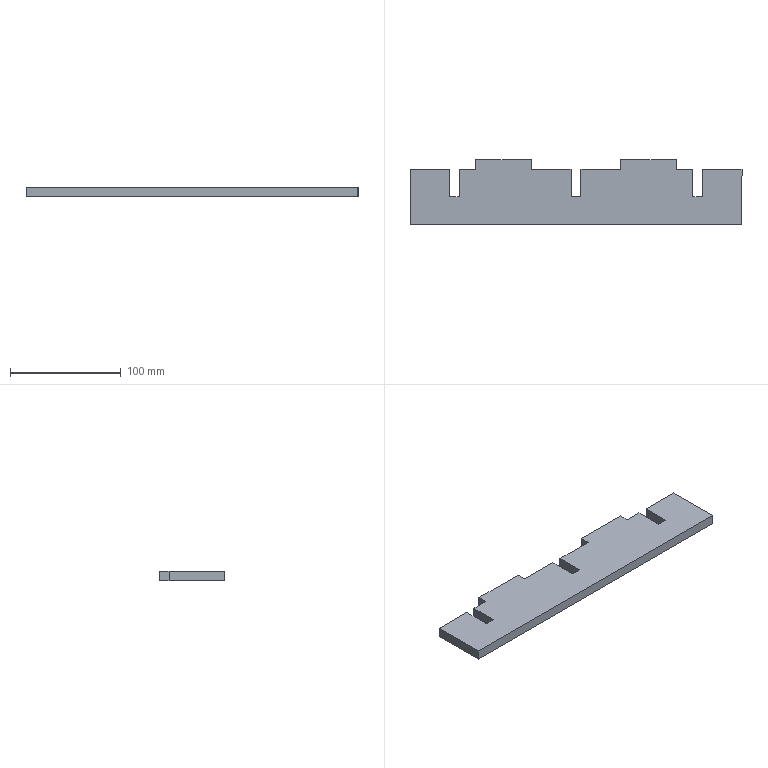Part | SolidWorks | features FlatPattern 1, SMBaseFlange 1, SheetMetal 1 | 1 solid | 26 faces | box 300 x 58.5 x 9 mm | volume 136575 mm3 | plane 26
STEP:
#1=CARTESIAN_POINT('',(743.25,-119.303,0.));
#2=VERTEX_POINT('',#1);
#3=CARTESIAN_POINT('',(743.25,-169.303,0.));
#4=VERTEX_POINT('',#3);
#5=CARTESIAN_POINT('',(743.25,-119.303,0.));
#6=DIRECTION('',(0.,-1.,0.));
#7=VECTOR('',#6,1000.);
#8=LINE('',#5,#7);
#9=EDGE_CURVE('',#2,#4,#8,.T.);
#10=ORIENTED_EDGE('',*,*,#9,.F.);
#11=CARTESIAN_POINT('',(743.25,-119.303,-9.));
#12=VERTEX_POINT('',#11);
#13=CARTESIAN_POINT('',(743.25,-119.303,-9.));
#14=DIRECTION('',(0.,0.,1.));
#15=VECTOR('',#14,1000.);
#16=LINE('',#13,#15);
#17=EDGE_CURVE('',#12,#2,#16,.T.);
#18=ORIENTED_EDGE('',*,*,#17,.F.);
#19=CARTESIAN_POINT('',(743.25,-169.303,-9.));
#20=VERTEX_POINT('',#19);
#21=CARTESIAN_POINT('',(743.25,-119.303,-9.));
#22=DIRECTION('',(0.,-1.,0.));
#23=VECTOR('',#22,1000.);
#24=LINE('',#21,#23);
#25=EDGE_CURVE('',#12,#20,#24,.T.);
#26=ORIENTED_EDGE('',*,*,#25,.T.);
#27=CARTESIAN_POINT('',(743.25,-169.303,-9.));
#28=DIRECTION('',(0.,0.,1.));
#29=VECTOR('',#28,1000.);
#30=LINE('',#27,#29);
#31=EDGE_CURVE('',#20,#4,#30,.T.);
#32=ORIENTED_EDGE('',*,*,#31,.T.);
#33=EDGE_LOOP('',(#10,#18,#26,#32));
#34=FACE_OUTER_BOUND('',#33,.T.);
#35=CARTESIAN_POINT('',(743.25,-119.303,-9.));
#36=DIRECTION('',(-1.,0.,0.));
#37=DIRECTION('',(0.,-1.,0.));
#38=AXIS2_PLACEMENT_3D('',#35,#36,#37);
#39=PLANE('',#38);
#40=ADVANCED_FACE('',(#34),#39,.T.);
#41=CARTESIAN_POINT('',(778.75,-119.303,0.));
#42=VERTEX_POINT('',#41);
#43=CARTESIAN_POINT('',(743.25,-119.303,0.));
#44=DIRECTION('',(-1.,0.,0.));
#45=VECTOR('',#44,1000.);
#46=LINE('',#43,#45);
#47=EDGE_CURVE('',#42,#2,#46,.T.);
#48=ORIENTED_EDGE('',*,*,#47,.F.);
#49=CARTESIAN_POINT('',(778.75,-119.303,-9.));
#50=VERTEX_POINT('',#49);
#51=CARTESIAN_POINT('',(778.75,-119.303,-9.));
#52=DIRECTION('',(0.,0.,1.));
#53=VECTOR('',#52,1000.);
#54=LINE('',#51,#53);
#55=EDGE_CURVE('',#50,#42,#54,.T.);
#56=ORIENTED_EDGE('',*,*,#55,.F.);
#57=CARTESIAN_POINT('',(743.25,-119.303,-9.));
#58=DIRECTION('',(-1.,0.,0.));
#59=VECTOR('',#58,1000.);
#60=LINE('',#57,#59);
#61=EDGE_CURVE('',#50,#12,#60,.T.);
#62=ORIENTED_EDGE('',*,*,#61,.T.);
#63=ORIENTED_EDGE('',*,*,#17,.T.);
#64=EDGE_LOOP('',(#48,#56,#62,#63));
#65=FACE_OUTER_BOUND('',#64,.T.);
#66=CARTESIAN_POINT('',(743.25,-119.303,-9.));
#67=DIRECTION('',(0.,1.,0.));
#68=DIRECTION('',(-1.,0.,0.));
#69=AXIS2_PLACEMENT_3D('',#66,#67,#68);
#70=PLANE('',#69);
#71=ADVANCED_FACE('',(#65),#70,.T.);
#72=CARTESIAN_POINT('',(778.75,-144.303,0.));
#73=VERTEX_POINT('',#72);
#74=CARTESIAN_POINT('',(778.75,-144.303,0.));
#75=DIRECTION('',(0.,1.,0.));
#76=VECTOR('',#75,1000.);
#77=LINE('',#74,#76);
#78=EDGE_CURVE('',#73,#42,#77,.T.);
#79=ORIENTED_EDGE('',*,*,#78,.F.);
#80=CARTESIAN_POINT('',(778.75,-144.303,-9.));
#81=VERTEX_POINT('',#80);
#82=CARTESIAN_POINT('',(778.75,-144.303,-9.));
#83=DIRECTION('',(0.,0.,1.));
#84=VECTOR('',#83,1000.);
#85=LINE('',#82,#84);
#86=EDGE_CURVE('',#81,#73,#85,.T.);
#87=ORIENTED_EDGE('',*,*,#86,.F.);
#88=CARTESIAN_POINT('',(778.75,-144.303,-9.));
#89=DIRECTION('',(0.,1.,0.));
#90=VECTOR('',#89,1000.);
#91=LINE('',#88,#90);
#92=EDGE_CURVE('',#81,#50,#91,.T.);
#93=ORIENTED_EDGE('',*,*,#92,.T.);
#94=ORIENTED_EDGE('',*,*,#55,.T.);
#95=EDGE_LOOP('',(#79,#87,#93,#94));
#96=FACE_OUTER_BOUND('',#95,.T.);
#97=CARTESIAN_POINT('',(778.75,-144.303,-9.));
#98=DIRECTION('',(1.,0.,0.));
#99=DIRECTION('',(0.,1.,0.));
#100=AXIS2_PLACEMENT_3D('',#97,#98,#99);
#101=PLANE('',#100);
#102=ADVANCED_FACE('',(#96),#101,.T.);
#103=CARTESIAN_POINT('',(787.75,-144.303,0.));
#104=VERTEX_POINT('',#103);
#105=CARTESIAN_POINT('',(787.75,-144.303,0.));
#106=DIRECTION('',(-1.,0.,0.));
#107=VECTOR('',#106,1000.);
#108=LINE('',#105,#107);
#109=EDGE_CURVE('',#104,#73,#108,.T.);
#110=ORIENTED_EDGE('',*,*,#109,.F.);
#111=CARTESIAN_POINT('',(787.75,-144.303,-9.));
#112=VERTEX_POINT('',#111);
#113=CARTESIAN_POINT('',(787.75,-144.303,-9.));
#114=DIRECTION('',(0.,0.,1.));
#115=VECTOR('',#114,1000.);
#116=LINE('',#113,#115);
#117=EDGE_CURVE('',#112,#104,#116,.T.);
#118=ORIENTED_EDGE('',*,*,#117,.F.);
#119=CARTESIAN_POINT('',(787.75,-144.303,-9.));
#120=DIRECTION('',(-1.,0.,0.));
#121=VECTOR('',#120,1000.);
#122=LINE('',#119,#121);
#123=EDGE_CURVE('',#112,#81,#122,.T.);
#124=ORIENTED_EDGE('',*,*,#123,.T.);
#125=ORIENTED_EDGE('',*,*,#86,.T.);
#126=EDGE_LOOP('',(#110,#118,#124,#125));
#127=FACE_OUTER_BOUND('',#126,.T.);
#128=CARTESIAN_POINT('',(787.75,-144.303,-9.));
#129=DIRECTION('',(0.,1.,0.));
#130=DIRECTION('',(0.,0.,1.));
#131=AXIS2_PLACEMENT_3D('',#128,#129,#130);
#132=PLANE('',#131);
#133=ADVANCED_FACE('',(#127),#132,.T.);
#134=CARTESIAN_POINT('',(787.75,-119.303,0.));
#135=VERTEX_POINT('',#134);
#136=CARTESIAN_POINT('',(787.75,-119.303,0.));
#137=DIRECTION('',(0.,-1.,0.));
#138=VECTOR('',#137,1000.);
#139=LINE('',#136,#138);
#140=EDGE_CURVE('',#135,#104,#139,.T.);
#141=ORIENTED_EDGE('',*,*,#140,.F.);
#142=CARTESIAN_POINT('',(787.75,-119.303,-9.));
#143=VERTEX_POINT('',#142);
#144=CARTESIAN_POINT('',(787.75,-119.303,-9.));
#145=DIRECTION('',(0.,0.,1.));
#146=VECTOR('',#145,1000.);
#147=LINE('',#144,#146);
#148=EDGE_CURVE('',#143,#135,#147,.T.);
#149=ORIENTED_EDGE('',*,*,#148,.F.);
#150=CARTESIAN_POINT('',(787.75,-119.303,-9.));
#151=DIRECTION('',(0.,-1.,0.));
#152=VECTOR('',#151,1000.);
#153=LINE('',#150,#152);
#154=EDGE_CURVE('',#143,#112,#153,.T.);
#155=ORIENTED_EDGE('',*,*,#154,.T.);
#156=ORIENTED_EDGE('',*,*,#117,.T.);
#157=EDGE_LOOP('',(#141,#149,#155,#156));
#158=FACE_OUTER_BOUND('',#157,.T.);
#159=CARTESIAN_POINT('',(787.75,-119.303,-9.));
#160=DIRECTION('',(-1.,0.,0.));
#161=DIRECTION('',(0.,-1.,0.));
#162=AXIS2_PLACEMENT_3D('',#159,#160,#161);
#163=PLANE('',#162);
#164=ADVANCED_FACE('',(#158),#163,.T.);
#165=CARTESIAN_POINT('',(802.75,-119.303,0.));
#166=VERTEX_POINT('',#165);
#167=CARTESIAN_POINT('',(787.75,-119.303,0.));
#168=DIRECTION('',(-1.,0.,0.));
#169=VECTOR('',#168,1000.);
#170=LINE('',#167,#169);
#171=EDGE_CURVE('',#166,#135,#170,.T.);
#172=ORIENTED_EDGE('',*,*,#171,.F.);
#173=CARTESIAN_POINT('',(802.75,-119.303,-9.));
#174=VERTEX_POINT('',#173);
#175=CARTESIAN_POINT('',(802.75,-119.303,-9.));
#176=DIRECTION('',(0.,0.,1.));
#177=VECTOR('',#176,1000.);
#178=LINE('',#175,#177);
#179=EDGE_CURVE('',#174,#166,#178,.T.);
#180=ORIENTED_EDGE('',*,*,#179,.F.);
#181=CARTESIAN_POINT('',(787.75,-119.303,-9.));
#182=DIRECTION('',(-1.,0.,0.));
#183=VECTOR('',#182,1000.);
#184=LINE('',#181,#183);
#185=EDGE_CURVE('',#174,#143,#184,.T.);
#186=ORIENTED_EDGE('',*,*,#185,.T.);
#187=ORIENTED_EDGE('',*,*,#148,.T.);
#188=EDGE_LOOP('',(#172,#180,#186,#187));
#189=FACE_OUTER_BOUND('',#188,.T.);
#190=CARTESIAN_POINT('',(787.75,-119.303,-9.));
#191=DIRECTION('',(0.,1.,0.));
#192=DIRECTION('',(-1.,0.,0.));
#193=AXIS2_PLACEMENT_3D('',#190,#191,#192);
#194=PLANE('',#193);
#195=ADVANCED_FACE('',(#189),#194,.T.);
#196=CARTESIAN_POINT('',(802.75,-110.803,0.));
#197=VERTEX_POINT('',#196);
#198=CARTESIAN_POINT('',(802.75,-119.303,0.));
#199=DIRECTION('',(0.,-1.,0.));
#200=VECTOR('',#199,1000.);
#201=LINE('',#198,#200);
#202=EDGE_CURVE('',#197,#166,#201,.T.);
#203=ORIENTED_EDGE('',*,*,#202,.F.);
#204=CARTESIAN_POINT('',(802.75,-110.803,-9.));
#205=VERTEX_POINT('',#204);
#206=CARTESIAN_POINT('',(802.75,-110.803,-9.));
#207=DIRECTION('',(0.,0.,1.));
#208=VECTOR('',#207,1000.);
#209=LINE('',#206,#208);
#210=EDGE_CURVE('',#205,#197,#209,.T.);
#211=ORIENTED_EDGE('',*,*,#210,.F.);
#212=CARTESIAN_POINT('',(802.75,-119.303,-9.));
#213=DIRECTION('',(0.,-1.,0.));
#214=VECTOR('',#213,1000.);
#215=LINE('',#212,#214);
#216=EDGE_CURVE('',#205,#174,#215,.T.);
#217=ORIENTED_EDGE('',*,*,#216,.T.);
#218=ORIENTED_EDGE('',*,*,#179,.T.);
#219=EDGE_LOOP('',(#203,#211,#217,#218));
#220=FACE_OUTER_BOUND('',#219,.T.);
#221=CARTESIAN_POINT('',(802.75,-119.303,-9.));
#222=DIRECTION('',(-1.,0.,0.));
#223=DIRECTION('',(0.,0.,1.));
#224=AXIS2_PLACEMENT_3D('',#221,#222,#223);
#225=PLANE('',#224);
#226=ADVANCED_FACE('',(#220),#225,.T.);
#227=CARTESIAN_POINT('',(852.75,-110.803,0.));
#228=VERTEX_POINT('',#227);
#229=CARTESIAN_POINT('',(802.75,-110.803,0.));
#230=DIRECTION('',(-1.,0.,0.));
#231=VECTOR('',#230,1000.);
#232=LINE('',#229,#231);
#233=EDGE_CURVE('',#228,#197,#232,.T.);
#234=ORIENTED_EDGE('',*,*,#233,.F.);
#235=CARTESIAN_POINT('',(852.75,-110.803,-9.));
#236=VERTEX_POINT('',#235);
#237=CARTESIAN_POINT('',(852.75,-110.803,-9.));
#238=DIRECTION('',(0.,0.,1.));
#239=VECTOR('',#238,1000.);
#240=LINE('',#237,#239);
#241=EDGE_CURVE('',#236,#228,#240,.T.);
#242=ORIENTED_EDGE('',*,*,#241,.F.);
#243=CARTESIAN_POINT('',(802.75,-110.803,-9.));
#244=DIRECTION('',(-1.,0.,0.));
#245=VECTOR('',#244,1000.);
#246=LINE('',#243,#245);
#247=EDGE_CURVE('',#236,#205,#246,.T.);
#248=ORIENTED_EDGE('',*,*,#247,.T.);
#249=ORIENTED_EDGE('',*,*,#210,.T.);
#250=EDGE_LOOP('',(#234,#242,#248,#249));
#251=FACE_OUTER_BOUND('',#250,.T.);
#252=CARTESIAN_POINT('',(802.75,-110.803,-9.));
#253=DIRECTION('',(0.,1.,0.));
#254=DIRECTION('',(0.,0.,1.));
#255=AXIS2_PLACEMENT_3D('',#252,#253,#254);
#256=PLANE('',#255);
#257=ADVANCED_FACE('',(#251),#256,.T.);
#258=CARTESIAN_POINT('',(852.75,-119.303,0.));
#259=VERTEX_POINT('',#258);
#260=CARTESIAN_POINT('',(852.75,-110.803,0.));
#261=DIRECTION('',(0.,1.,0.));
#262=VECTOR('',#261,1000.);
#263=LINE('',#260,#262);
#264=EDGE_CURVE('',#259,#228,#263,.T.);
#265=ORIENTED_EDGE('',*,*,#264,.F.);
#266=CARTESIAN_POINT('',(852.75,-119.303,-9.));
#267=VERTEX_POINT('',#266);
#268=CARTESIAN_POINT('',(852.75,-119.303,-9.));
#269=DIRECTION('',(0.,0.,1.));
#270=VECTOR('',#269,1000.);
#271=LINE('',#268,#270);
#272=EDGE_CURVE('',#267,#259,#271,.T.);
#273=ORIENTED_EDGE('',*,*,#272,.F.);
#274=CARTESIAN_POINT('',(852.75,-110.803,-9.));
#275=DIRECTION('',(0.,1.,0.));
#276=VECTOR('',#275,1000.);
#277=LINE('',#274,#276);
#278=EDGE_CURVE('',#267,#236,#277,.T.);
#279=ORIENTED_EDGE('',*,*,#278,.T.);
#280=ORIENTED_EDGE('',*,*,#241,.T.);
#281=EDGE_LOOP('',(#265,#273,#279,#280));
#282=FACE_OUTER_BOUND('',#281,.T.);
#283=CARTESIAN_POINT('',(852.75,-110.803,-9.));
#284=DIRECTION('',(1.,0.,0.));
#285=DIRECTION('',(0.,0.,-1.));
#286=AXIS2_PLACEMENT_3D('',#283,#284,#285);
#287=PLANE('',#286);
#288=ADVANCED_FACE('',(#282),#287,.T.);
#289=CARTESIAN_POINT('',(888.75,-119.303,0.));
#290=VERTEX_POINT('',#289);
#291=CARTESIAN_POINT('',(852.75,-119.303,0.));
#292=DIRECTION('',(-1.,0.,0.));
#293=VECTOR('',#292,1000.);
#294=LINE('',#291,#293);
#295=EDGE_CURVE('',#290,#259,#294,.T.);
#296=ORIENTED_EDGE('',*,*,#295,.F.);
#297=CARTESIAN_POINT('',(888.75,-119.303,-9.));
#298=VERTEX_POINT('',#297);
#299=CARTESIAN_POINT('',(888.75,-119.303,-9.));
#300=DIRECTION('',(0.,0.,1.));
#301=VECTOR('',#300,1000.);
#302=LINE('',#299,#301);
#303=EDGE_CURVE('',#298,#290,#302,.T.);
#304=ORIENTED_EDGE('',*,*,#303,.F.);
#305=CARTESIAN_POINT('',(852.75,-119.303,-9.));
#306=DIRECTION('',(-1.,0.,0.));
#307=VECTOR('',#306,1000.);
#308=LINE('',#305,#307);
#309=EDGE_CURVE('',#298,#267,#308,.T.);
#310=ORIENTED_EDGE('',*,*,#309,.T.);
#311=ORIENTED_EDGE('',*,*,#272,.T.);
#312=EDGE_LOOP('',(#296,#304,#310,#311));
#313=FACE_OUTER_BOUND('',#312,.T.);
#314=CARTESIAN_POINT('',(852.75,-119.303,-9.));
#315=DIRECTION('',(0.,1.,0.));
#316=DIRECTION('',(-1.,0.,0.));
#317=AXIS2_PLACEMENT_3D('',#314,#315,#316);
#318=PLANE('',#317);
#319=ADVANCED_FACE('',(#313),#318,.T.);
#320=CARTESIAN_POINT('',(888.75,-144.303,0.));
#321=VERTEX_POINT('',#320);
#322=CARTESIAN_POINT('',(888.75,-144.303,0.));
#323=DIRECTION('',(0.,1.,0.));
#324=VECTOR('',#323,1000.);
#325=LINE('',#322,#324);
#326=EDGE_CURVE('',#321,#290,#325,.T.);
#327=ORIENTED_EDGE('',*,*,#326,.F.);
#328=CARTESIAN_POINT('',(888.75,-144.303,-9.));
#329=VERTEX_POINT('',#328);
#330=CARTESIAN_POINT('',(888.75,-144.303,-9.));
#331=DIRECTION('',(0.,0.,1.));
#332=VECTOR('',#331,1000.);
#333=LINE('',#330,#332);
#334=EDGE_CURVE('',#329,#321,#333,.T.);
#335=ORIENTED_EDGE('',*,*,#334,.F.);
#336=CARTESIAN_POINT('',(888.75,-144.303,-9.));
#337=DIRECTION('',(0.,1.,0.));
#338=VECTOR('',#337,1000.);
#339=LINE('',#336,#338);
#340=EDGE_CURVE('',#329,#298,#339,.T.);
#341=ORIENTED_EDGE('',*,*,#340,.T.);
#342=ORIENTED_EDGE('',*,*,#303,.T.);
#343=EDGE_LOOP('',(#327,#335,#341,#342));
#344=FACE_OUTER_BOUND('',#343,.T.);
#345=CARTESIAN_POINT('',(888.75,-144.303,-9.));
#346=DIRECTION('',(1.,0.,0.));
#347=DIRECTION('',(0.,1.,0.));
#348=AXIS2_PLACEMENT_3D('',#345,#346,#347);
#349=PLANE('',#348);
#350=ADVANCED_FACE('',(#344),#349,.T.);
#351=CARTESIAN_POINT('',(897.75,-144.303,0.));
#352=VERTEX_POINT('',#351);
#353=CARTESIAN_POINT('',(897.75,-144.303,0.));
#354=DIRECTION('',(-1.,0.,0.));
#355=VECTOR('',#354,1000.);
#356=LINE('',#353,#355);
#357=EDGE_CURVE('',#352,#321,#356,.T.);
#358=ORIENTED_EDGE('',*,*,#357,.F.);
#359=CARTESIAN_POINT('',(897.75,-144.303,-9.));
#360=VERTEX_POINT('',#359);
#361=CARTESIAN_POINT('',(897.75,-144.303,-9.));
#362=DIRECTION('',(0.,0.,1.));
#363=VECTOR('',#362,1000.);
#364=LINE('',#361,#363);
#365=EDGE_CURVE('',#360,#352,#364,.T.);
#366=ORIENTED_EDGE('',*,*,#365,.F.);
#367=CARTESIAN_POINT('',(897.75,-144.303,-9.));
#368=DIRECTION('',(-1.,0.,0.));
#369=VECTOR('',#368,1000.);
#370=LINE('',#367,#369);
#371=EDGE_CURVE('',#360,#329,#370,.T.);
#372=ORIENTED_EDGE('',*,*,#371,.T.);
#373=ORIENTED_EDGE('',*,*,#334,.T.);
#374=EDGE_LOOP('',(#358,#366,#372,#373));
#375=FACE_OUTER_BOUND('',#374,.T.);
#376=CARTESIAN_POINT('',(897.75,-144.303,-9.));
#377=DIRECTION('',(0.,1.,0.));
#378=DIRECTION('',(0.,0.,1.));
#379=AXIS2_PLACEMENT_3D('',#376,#377,#378);
#380=PLANE('',#379);
#381=ADVANCED_FACE('',(#375),#380,.T.);
#382=CARTESIAN_POINT('',(897.75,-119.303,0.));
#383=VERTEX_POINT('',#382);
#384=CARTESIAN_POINT('',(897.75,-119.303,0.));
#385=DIRECTION('',(0.,-1.,0.));
#386=VECTOR('',#385,1000.);
#387=LINE('',#384,#386);
#388=EDGE_CURVE('',#383,#352,#387,.T.);
#389=ORIENTED_EDGE('',*,*,#388,.F.);
#390=CARTESIAN_POINT('',(897.75,-119.303,-9.));
#391=VERTEX_POINT('',#390);
#392=CARTESIAN_POINT('',(897.75,-119.303,-9.));
#393=DIRECTION('',(0.,0.,1.));
#394=VECTOR('',#393,1000.);
#395=LINE('',#392,#394);
#396=EDGE_CURVE('',#391,#383,#395,.T.);
#397=ORIENTED_EDGE('',*,*,#396,.F.);
#398=CARTESIAN_POINT('',(897.75,-119.303,-9.));
#399=DIRECTION('',(0.,-1.,0.));
#400=VECTOR('',#399,1000.);
#401=LINE('',#398,#400);
#402=EDGE_CURVE('',#391,#360,#401,.T.);
#403=ORIENTED_EDGE('',*,*,#402,.T.);
#404=ORIENTED_EDGE('',*,*,#365,.T.);
#405=EDGE_LOOP('',(#389,#397,#403,#404));
#406=FACE_OUTER_BOUND('',#405,.T.);
#407=CARTESIAN_POINT('',(897.75,-119.303,-9.));
#408=DIRECTION('',(-1.,0.,0.));
#409=DIRECTION('',(0.,-1.,0.));
#410=AXIS2_PLACEMENT_3D('',#407,#408,#409);
#411=PLANE('',#410);
#412=ADVANCED_FACE('',(#406),#411,.T.);
#413=CARTESIAN_POINT('',(933.75,-119.303,0.));
#414=VERTEX_POINT('',#413);
#415=CARTESIAN_POINT('',(897.75,-119.303,0.));
#416=DIRECTION('',(-1.,0.,0.));
#417=VECTOR('',#416,1000.);
#418=LINE('',#415,#417);
#419=EDGE_CURVE('',#414,#383,#418,.T.);
#420=ORIENTED_EDGE('',*,*,#419,.F.);
#421=CARTESIAN_POINT('',(933.75,-119.303,-9.));
#422=VERTEX_POINT('',#421);
#423=CARTESIAN_POINT('',(933.75,-119.303,-9.));
#424=DIRECTION('',(0.,0.,1.));
#425=VECTOR('',#424,1000.);
#426=LINE('',#423,#425);
#427=EDGE_CURVE('',#422,#414,#426,.T.);
#428=ORIENTED_EDGE('',*,*,#427,.F.);
#429=CARTESIAN_POINT('',(897.75,-119.303,-9.));
#430=DIRECTION('',(-1.,0.,0.));
#431=VECTOR('',#430,1000.);
#432=LINE('',#429,#431);
#433=EDGE_CURVE('',#422,#391,#432,.T.);
#434=ORIENTED_EDGE('',*,*,#433,.T.);
#435=ORIENTED_EDGE('',*,*,#396,.T.);
#436=EDGE_LOOP('',(#420,#428,#434,#435));
#437=FACE_OUTER_BOUND('',#436,.T.);
#438=CARTESIAN_POINT('',(897.75,-119.303,-9.));
#439=DIRECTION('',(0.,1.,0.));
#440=DIRECTION('',(-1.,0.,0.));
#441=AXIS2_PLACEMENT_3D('',#438,#439,#440);
#442=PLANE('',#441);
#443=ADVANCED_FACE('',(#437),#442,.T.);
#444=CARTESIAN_POINT('',(933.75,-110.803,0.));
#445=VERTEX_POINT('',#444);
#446=CARTESIAN_POINT('',(933.75,-110.803,0.));
#447=DIRECTION('',(0.,-1.,0.));
#448=VECTOR('',#447,1000.);
#449=LINE('',#446,#448);
#450=EDGE_CURVE('',#445,#414,#449,.T.);
#451=ORIENTED_EDGE('',*,*,#450,.F.);
#452=CARTESIAN_POINT('',(933.75,-110.803,-9.));
#453=VERTEX_POINT('',#452);
#454=CARTESIAN_POINT('',(933.75,-110.803,-9.));
#455=DIRECTION('',(0.,0.,1.));
#456=VECTOR('',#455,1000.);
#457=LINE('',#454,#456);
#458=EDGE_CURVE('',#453,#445,#457,.T.);
#459=ORIENTED_EDGE('',*,*,#458,.F.);
#460=CARTESIAN_POINT('',(933.75,-110.803,-9.));
#461=DIRECTION('',(0.,-1.,0.));
#462=VECTOR('',#461,1000.);
#463=LINE('',#460,#462);
#464=EDGE_CURVE('',#453,#422,#463,.T.);
#465=ORIENTED_EDGE('',*,*,#464,.T.);
#466=ORIENTED_EDGE('',*,*,#427,.T.);
#467=EDGE_LOOP('',(#451,#459,#465,#466));
#468=FACE_OUTER_BOUND('',#467,.T.);
#469=CARTESIAN_POINT('',(933.75,-110.803,-9.));
#470=DIRECTION('',(-1.,0.,0.));
#471=DIRECTION('',(0.,0.,1.));
#472=AXIS2_PLACEMENT_3D('',#469,#470,#471);
#473=PLANE('',#472);
#474=ADVANCED_FACE('',(#468),#473,.T.);
#475=CARTESIAN_POINT('',(983.75,-110.803,0.));
#476=VERTEX_POINT('',#475);
#477=CARTESIAN_POINT('',(983.75,-110.803,0.));
#478=DIRECTION('',(-1.,0.,0.));
#479=VECTOR('',#478,1000.);
#480=LINE('',#477,#479);
#481=EDGE_CURVE('',#476,#445,#480,.T.);
#482=ORIENTED_EDGE('',*,*,#481,.F.);
#483=CARTESIAN_POINT('',(983.75,-110.803,-9.));
#484=VERTEX_POINT('',#483);
#485=CARTESIAN_POINT('',(983.75,-110.803,-9.));
#486=DIRECTION('',(0.,0.,1.));
#487=VECTOR('',#486,1000.);
#488=LINE('',#485,#487);
#489=EDGE_CURVE('',#484,#476,#488,.T.);
#490=ORIENTED_EDGE('',*,*,#489,.F.);
#491=CARTESIAN_POINT('',(983.75,-110.803,-9.));
#492=DIRECTION('',(-1.,0.,0.));
#493=VECTOR('',#492,1000.);
#494=LINE('',#491,#493);
#495=EDGE_CURVE('',#484,#453,#494,.T.);
#496=ORIENTED_EDGE('',*,*,#495,.T.);
#497=ORIENTED_EDGE('',*,*,#458,.T.);
#498=EDGE_LOOP('',(#482,#490,#496,#497));
#499=FACE_OUTER_BOUND('',#498,.T.);
#500=CARTESIAN_POINT('',(983.75,-110.803,-9.));
#501=DIRECTION('',(0.,1.,0.));
#502=DIRECTION('',(-1.,0.,0.));
#503=AXIS2_PLACEMENT_3D('',#500,#501,#502);
#504=PLANE('',#503);
#505=ADVANCED_FACE('',(#499),#504,.T.);
#506=CARTESIAN_POINT('',(983.75,-119.303,0.));
#507=VERTEX_POINT('',#506);
#508=CARTESIAN_POINT('',(983.75,-119.303,0.));
#509=DIRECTION('',(0.,1.,0.));
#510=VECTOR('',#509,1000.);
#511=LINE('',#508,#510);
#512=EDGE_CURVE('',#507,#476,#511,.T.);
#513=ORIENTED_EDGE('',*,*,#512,.F.);
#514=CARTESIAN_POINT('',(983.75,-119.303,-9.));
#515=VERTEX_POINT('',#514);
#516=CARTESIAN_POINT('',(983.75,-119.303,-9.));
#517=DIRECTION('',(0.,0.,1.));
#518=VECTOR('',#517,1000.);
#519=LINE('',#516,#518);
#520=EDGE_CURVE('',#515,#507,#519,.T.);
#521=ORIENTED_EDGE('',*,*,#520,.F.);
#522=CARTESIAN_POINT('',(983.75,-119.303,-9.));
#523=DIRECTION('',(0.,1.,0.));
#524=VECTOR('',#523,1000.);
#525=LINE('',#522,#524);
#526=EDGE_CURVE('',#515,#484,#525,.T.);
#527=ORIENTED_EDGE('',*,*,#526,.T.);
#528=ORIENTED_EDGE('',*,*,#489,.T.);
#529=EDGE_LOOP('',(#513,#521,#527,#528));
#530=FACE_OUTER_BOUND('',#529,.T.);
#531=CARTESIAN_POINT('',(983.75,-119.303,-9.));
#532=DIRECTION('',(1.,0.,0.));
#533=DIRECTION('',(0.,1.,0.));
#534=AXIS2_PLACEMENT_3D('',#531,#532,#533);
#535=PLANE('',#534);
#536=ADVANCED_FACE('',(#530),#535,.T.);
#537=CARTESIAN_POINT('',(998.75,-119.303,0.));
#538=VERTEX_POINT('',#537);
#539=CARTESIAN_POINT('',(983.75,-119.303,0.));
#540=DIRECTION('',(-1.,0.,0.));
#541=VECTOR('',#540,1000.);
#542=LINE('',#539,#541);
#543=EDGE_CURVE('',#538,#507,#542,.T.);
#544=ORIENTED_EDGE('',*,*,#543,.F.);
#545=CARTESIAN_POINT('',(998.75,-119.303,-9.));
#546=VERTEX_POINT('',#545);
#547=CARTESIAN_POINT('',(998.75,-119.303,-9.));
#548=DIRECTION('',(0.,0.,1.));
#549=VECTOR('',#548,1000.);
#550=LINE('',#547,#549);
#551=EDGE_CURVE('',#546,#538,#550,.T.);
#552=ORIENTED_EDGE('',*,*,#551,.F.);
#553=CARTESIAN_POINT('',(983.75,-119.303,-9.));
#554=DIRECTION('',(-1.,0.,0.));
#555=VECTOR('',#554,1000.);
#556=LINE('',#553,#555);
#557=EDGE_CURVE('',#546,#515,#556,.T.);
#558=ORIENTED_EDGE('',*,*,#557,.T.);
#559=ORIENTED_EDGE('',*,*,#520,.T.);
#560=EDGE_LOOP('',(#544,#552,#558,#559));
#561=FACE_OUTER_BOUND('',#560,.T.);
#562=CARTESIAN_POINT('',(983.75,-119.303,-9.));
#563=DIRECTION('',(0.,1.,0.));
#564=DIRECTION('',(-1.,0.,0.));
#565=AXIS2_PLACEMENT_3D('',#562,#563,#564);
#566=PLANE('',#565);
#567=ADVANCED_FACE('',(#561),#566,.T.);
#568=CARTESIAN_POINT('',(998.75,-144.303,0.));
#569=VERTEX_POINT('',#568);
#570=CARTESIAN_POINT('',(998.75,-144.303,0.));
#571=DIRECTION('',(0.,1.,0.));
#572=VECTOR('',#571,1000.);
#573=LINE('',#570,#572);
#574=EDGE_CURVE('',#569,#538,#573,.T.);
#575=ORIENTED_EDGE('',*,*,#574,.F.);
#576=CARTESIAN_POINT('',(998.75,-144.303,-9.));
#577=VERTEX_POINT('',#576);
#578=CARTESIAN_POINT('',(998.75,-144.303,-9.));
#579=DIRECTION('',(0.,0.,1.));
#580=VECTOR('',#579,1000.);
#581=LINE('',#578,#580);
#582=EDGE_CURVE('',#577,#569,#581,.T.);
#583=ORIENTED_EDGE('',*,*,#582,.F.);
#584=CARTESIAN_POINT('',(998.75,-144.303,-9.));
#585=DIRECTION('',(0.,1.,0.));
#586=VECTOR('',#585,1000.);
#587=LINE('',#584,#586);
#588=EDGE_CURVE('',#577,#546,#587,.T.);
#589=ORIENTED_EDGE('',*,*,#588,.T.);
#590=ORIENTED_EDGE('',*,*,#551,.T.);
#591=EDGE_LOOP('',(#575,#583,#589,#590));
#592=FACE_OUTER_BOUND('',#591,.T.);
#593=CARTESIAN_POINT('',(998.75,-144.303,-9.));
#594=DIRECTION('',(1.,0.,0.));
#595=DIRECTION('',(0.,1.,0.));
#596=AXIS2_PLACEMENT_3D('',#593,#594,#595);
#597=PLANE('',#596);
#598=ADVANCED_FACE('',(#592),#597,.T.);
#599=CARTESIAN_POINT('',(1007.75,-144.303,0.));
#600=VERTEX_POINT('',#599);
#601=CARTESIAN_POINT('',(1007.75,-144.303,0.));
#602=DIRECTION('',(-1.,0.,0.));
#603=VECTOR('',#602,1000.);
#604=LINE('',#601,#603);
#605=EDGE_CURVE('',#600,#569,#604,.T.);
#606=ORIENTED_EDGE('',*,*,#605,.F.);
#607=CARTESIAN_POINT('',(1007.75,-144.303,-9.));
#608=VERTEX_POINT('',#607);
#609=CARTESIAN_POINT('',(1007.75,-144.303,-9.));
#610=DIRECTION('',(0.,0.,1.));
#611=VECTOR('',#610,1000.);
#612=LINE('',#609,#611);
#613=EDGE_CURVE('',#608,#600,#612,.T.);
#614=ORIENTED_EDGE('',*,*,#613,.F.);
#615=CARTESIAN_POINT('',(1007.75,-144.303,-9.));
#616=DIRECTION('',(-1.,0.,0.));
#617=VECTOR('',#616,1000.);
#618=LINE('',#615,#617);
#619=EDGE_CURVE('',#608,#577,#618,.T.);
#620=ORIENTED_EDGE('',*,*,#619,.T.);
#621=ORIENTED_EDGE('',*,*,#582,.T.);
#622=EDGE_LOOP('',(#606,#614,#620,#621));
#623=FACE_OUTER_BOUND('',#622,.T.);
#624=CARTESIAN_POINT('',(1007.75,-144.303,-9.));
#625=DIRECTION('',(0.,1.,0.));
#626=DIRECTION('',(0.,0.,1.));
#627=AXIS2_PLACEMENT_3D('',#624,#625,#626);
#628=PLANE('',#627);
#629=ADVANCED_FACE('',(#623),#628,.T.);
#630=CARTESIAN_POINT('',(1007.75,-119.303,0.));
#631=VERTEX_POINT('',#630);
#632=CARTESIAN_POINT('',(1007.75,-119.303,0.));
#633=DIRECTION('',(0.,-1.,0.));
#634=VECTOR('',#633,1000.);
#635=LINE('',#632,#634);
#636=EDGE_CURVE('',#631,#600,#635,.T.);
#637=ORIENTED_EDGE('',*,*,#636,.F.);
#638=CARTESIAN_POINT('',(1007.75,-119.303,-9.));
#639=VERTEX_POINT('',#638);
#640=CARTESIAN_POINT('',(1007.75,-119.303,-9.));
#641=DIRECTION('',(0.,0.,1.));
#642=VECTOR('',#641,1000.);
#643=LINE('',#640,#642);
#644=EDGE_CURVE('',#639,#631,#643,.T.);
#645=ORIENTED_EDGE('',*,*,#644,.F.);
#646=CARTESIAN_POINT('',(1007.75,-119.303,-9.));
#647=DIRECTION('',(0.,-1.,0.));
#648=VECTOR('',#647,1000.);
#649=LINE('',#646,#648);
#650=EDGE_CURVE('',#639,#608,#649,.T.);
#651=ORIENTED_EDGE('',*,*,#650,.T.);
#652=ORIENTED_EDGE('',*,*,#613,.T.);
#653=EDGE_LOOP('',(#637,#645,#651,#652));
#654=FACE_OUTER_BOUND('',#653,.T.);
#655=CARTESIAN_POINT('',(1007.75,-119.303,-9.));
#656=DIRECTION('',(-1.,0.,0.));
#657=DIRECTION('',(0.,-1.,0.));
#658=AXIS2_PLACEMENT_3D('',#655,#656,#657);
#659=PLANE('',#658);
#660=ADVANCED_FACE('',(#654),#659,.T.);
#661=CARTESIAN_POINT('',(1043.25,-119.303,0.));
#662=VERTEX_POINT('',#661);
#663=CARTESIAN_POINT('',(1007.75,-119.303,0.));
#664=DIRECTION('',(-1.,0.,0.));
#665=VECTOR('',#664,1000.);
#666=LINE('',#663,#665);
#667=EDGE_CURVE('',#662,#631,#666,.T.);
#668=ORIENTED_EDGE('',*,*,#667,.F.);
#669=CARTESIAN_POINT('',(1043.25,-119.303,-9.));
#670=VERTEX_POINT('',#669);
#671=CARTESIAN_POINT('',(1043.25,-119.303,-9.));
#672=DIRECTION('',(0.,0.,1.));
#673=VECTOR('',#672,1000.);
#674=LINE('',#671,#673);
#675=EDGE_CURVE('',#670,#662,#674,.T.);
#676=ORIENTED_EDGE('',*,*,#675,.F.);
#677=CARTESIAN_POINT('',(1007.75,-119.303,-9.));
#678=DIRECTION('',(-1.,0.,0.));
#679=VECTOR('',#678,1000.);
#680=LINE('',#677,#679);
#681=EDGE_CURVE('',#670,#639,#680,.T.);
#682=ORIENTED_EDGE('',*,*,#681,.T.);
#683=ORIENTED_EDGE('',*,*,#644,.T.);
#684=EDGE_LOOP('',(#668,#676,#682,#683));
#685=FACE_OUTER_BOUND('',#684,.T.);
#686=CARTESIAN_POINT('',(1007.75,-119.303,-9.));
#687=DIRECTION('',(0.,1.,0.));
#688=DIRECTION('',(-1.,0.,0.));
#689=AXIS2_PLACEMENT_3D('',#686,#687,#688);
#690=PLANE('',#689);
#691=ADVANCED_FACE('',(#685),#690,.T.);
#692=CARTESIAN_POINT('',(1043.25,-169.303,0.));
#693=VERTEX_POINT('',#692);
#694=CARTESIAN_POINT('',(1043.25,-119.303,0.));
#695=DIRECTION('',(0.,1.,0.));
#696=VECTOR('',#695,1000.);
#697=LINE('',#694,#696);
#698=EDGE_CURVE('',#693,#662,#697,.T.);
#699=ORIENTED_EDGE('',*,*,#698,.F.);
#700=CARTESIAN_POINT('',(1043.25,-169.303,-9.));
#701=VERTEX_POINT('',#700);
#702=CARTESIAN_POINT('',(1043.25,-169.303,-9.));
#703=DIRECTION('',(0.,0.,1.));
#704=VECTOR('',#703,1000.);
#705=LINE('',#702,#704);
#706=EDGE_CURVE('',#701,#693,#705,.T.);
#707=ORIENTED_EDGE('',*,*,#706,.F.);
#708=CARTESIAN_POINT('',(1043.25,-119.303,-9.));
#709=DIRECTION('',(0.,1.,0.));
#710=VECTOR('',#709,1000.);
#711=LINE('',#708,#710);
#712=EDGE_CURVE('',#701,#670,#711,.T.);
#713=ORIENTED_EDGE('',*,*,#712,.T.);
#714=ORIENTED_EDGE('',*,*,#675,.T.);
#715=EDGE_LOOP('',(#699,#707,#713,#714));
#716=FACE_OUTER_BOUND('',#715,.T.);
#717=CARTESIAN_POINT('',(1043.25,-119.303,-9.));
#718=DIRECTION('',(1.,0.,0.));
#719=DIRECTION('',(0.,1.,0.));
#720=AXIS2_PLACEMENT_3D('',#717,#718,#719);
#721=PLANE('',#720);
#722=ADVANCED_FACE('',(#716),#721,.T.);
#723=CARTESIAN_POINT('',(743.25,-169.303,0.));
#724=DIRECTION('',(1.,0.,0.));
#725=VECTOR('',#724,1000.);
#726=LINE('',#723,#725);
#727=EDGE_CURVE('',#4,#693,#726,.T.);
#728=ORIENTED_EDGE('',*,*,#727,.F.);
#729=ORIENTED_EDGE('',*,*,#31,.F.);
#730=CARTESIAN_POINT('',(743.25,-169.303,-9.));
#731=DIRECTION('',(1.,0.,0.));
#732=VECTOR('',#731,1000.);
#733=LINE('',#730,#732);
#734=EDGE_CURVE('',#20,#701,#733,.T.);
#735=ORIENTED_EDGE('',*,*,#734,.T.);
#736=ORIENTED_EDGE('',*,*,#706,.T.);
#737=EDGE_LOOP('',(#728,#729,#735,#736));
#738=FACE_OUTER_BOUND('',#737,.T.);
#739=CARTESIAN_POINT('',(743.25,-169.303,-9.));
#740=DIRECTION('',(0.,-1.,0.));
#741=DIRECTION('',(0.,0.,-1.));
#742=AXIS2_PLACEMENT_3D('',#739,#740,#741);
#743=PLANE('',#742);
#744=ADVANCED_FACE('',(#738),#743,.T.);
#745=ORIENTED_EDGE('',*,*,#25,.F.);
#746=ORIENTED_EDGE('',*,*,#61,.F.);
#747=ORIENTED_EDGE('',*,*,#92,.F.);
#748=ORIENTED_EDGE('',*,*,#123,.F.);
#749=ORIENTED_EDGE('',*,*,#154,.F.);
#750=ORIENTED_EDGE('',*,*,#185,.F.);
#751=ORIENTED_EDGE('',*,*,#216,.F.);
#752=ORIENTED_EDGE('',*,*,#247,.F.);
#753=ORIENTED_EDGE('',*,*,#278,.F.);
#754=ORIENTED_EDGE('',*,*,#309,.F.);
#755=ORIENTED_EDGE('',*,*,#340,.F.);
#756=ORIENTED_EDGE('',*,*,#371,.F.);
#757=ORIENTED_EDGE('',*,*,#402,.F.);
#758=ORIENTED_EDGE('',*,*,#433,.F.);
#759=ORIENTED_EDGE('',*,*,#464,.F.);
#760=ORIENTED_EDGE('',*,*,#495,.F.);
#761=ORIENTED_EDGE('',*,*,#526,.F.);
#762=ORIENTED_EDGE('',*,*,#557,.F.);
#763=ORIENTED_EDGE('',*,*,#588,.F.);
#764=ORIENTED_EDGE('',*,*,#619,.F.);
#765=ORIENTED_EDGE('',*,*,#650,.F.);
#766=ORIENTED_EDGE('',*,*,#681,.F.);
#767=ORIENTED_EDGE('',*,*,#712,.F.);
#768=ORIENTED_EDGE('',*,*,#734,.F.);
#769=EDGE_LOOP('',(#745,#746,#747,#748,#749,#750,#751,#752,#753,#754,#755,#756,#757,#758,#759,#760,#761,#762,#763,#764,#765,#766,#767,#768));
#770=FACE_OUTER_BOUND('',#769,.T.);
#771=CARTESIAN_POINT('',(0.,0.,-9.));
#772=DIRECTION('',(0.,0.,1.));
#773=DIRECTION('',(1.,0.,0.));
#774=AXIS2_PLACEMENT_3D('',#771,#772,#773);
#775=PLANE('',#774);
#776=ADVANCED_FACE('',(#770),#775,.F.);
#777=ORIENTED_EDGE('',*,*,#9,.T.);
#778=ORIENTED_EDGE('',*,*,#727,.T.);
#779=ORIENTED_EDGE('',*,*,#698,.T.);
#780=ORIENTED_EDGE('',*,*,#667,.T.);
#781=ORIENTED_EDGE('',*,*,#636,.T.);
#782=ORIENTED_EDGE('',*,*,#605,.T.);
#783=ORIENTED_EDGE('',*,*,#574,.T.);
#784=ORIENTED_EDGE('',*,*,#543,.T.);
#785=ORIENTED_EDGE('',*,*,#512,.T.);
#786=ORIENTED_EDGE('',*,*,#481,.T.);
#787=ORIENTED_EDGE('',*,*,#450,.T.);
#788=ORIENTED_EDGE('',*,*,#419,.T.);
#789=ORIENTED_EDGE('',*,*,#388,.T.);
#790=ORIENTED_EDGE('',*,*,#357,.T.);
#791=ORIENTED_EDGE('',*,*,#326,.T.);
#792=ORIENTED_EDGE('',*,*,#295,.T.);
#793=ORIENTED_EDGE('',*,*,#264,.T.);
#794=ORIENTED_EDGE('',*,*,#233,.T.);
#795=ORIENTED_EDGE('',*,*,#202,.T.);
#796=ORIENTED_EDGE('',*,*,#171,.T.);
#797=ORIENTED_EDGE('',*,*,#140,.T.);
#798=ORIENTED_EDGE('',*,*,#109,.T.);
#799=ORIENTED_EDGE('',*,*,#78,.T.);
#800=ORIENTED_EDGE('',*,*,#47,.T.);
#801=EDGE_LOOP('',(#777,#778,#779,#780,#781,#782,#783,#784,#785,#786,#787,#788,#789,#790,#791,#792,#793,#794,#795,#796,#797,#798,#799,#800));
#802=FACE_OUTER_BOUND('',#801,.T.);
#803=CARTESIAN_POINT('',(0.,0.,0.));
#804=DIRECTION('',(0.,0.,1.));
#805=DIRECTION('',(1.,0.,0.));
#806=AXIS2_PLACEMENT_3D('',#803,#804,#805);
#807=PLANE('',#806);
#808=ADVANCED_FACE('',(#802),#807,.T.);
#809=CLOSED_SHELL('',(#40,#71,#102,#133,#164,#195,#226,#257,#288,#319,#350,#381,#412,#443,#474,#505,#536,#567,#598,#629,#660,#691,#722,#744,#776,#808));
#810=MANIFOLD_SOLID_BREP('',#809);
#811=CARTESIAN_POINT('',(0.,0.,0.));
#812=DIRECTION('',(0.,0.,1.));
#813=DIRECTION('',(1.,0.,0.));
#814=AXIS2_PLACEMENT_3D('',#811,#812,#813);
#815=(LENGTH_UNIT()NAMED_UNIT(*)SI_UNIT(.MILLI.,.METRE.));
#816=UNCERTAINTY_MEASURE_WITH_UNIT(LENGTH_MEASURE(0.00001),#815,'','');
#817=(NAMED_UNIT(*)PLANE_ANGLE_UNIT()SI_UNIT($,.RADIAN.));
#818=(NAMED_UNIT(*)SI_UNIT($,.STERADIAN.)SOLID_ANGLE_UNIT());
#819=(GEOMETRIC_REPRESENTATION_CONTEXT(3)GLOBAL_UNCERTAINTY_ASSIGNED_CONTEXT((#816))GLOBAL_UNIT_ASSIGNED_CONTEXT((#815,#817,#818))REPRESENTATION_CONTEXT('',''));
#820=ADVANCED_BREP_SHAPE_REPRESENTATION('',(#810,#814),#819);